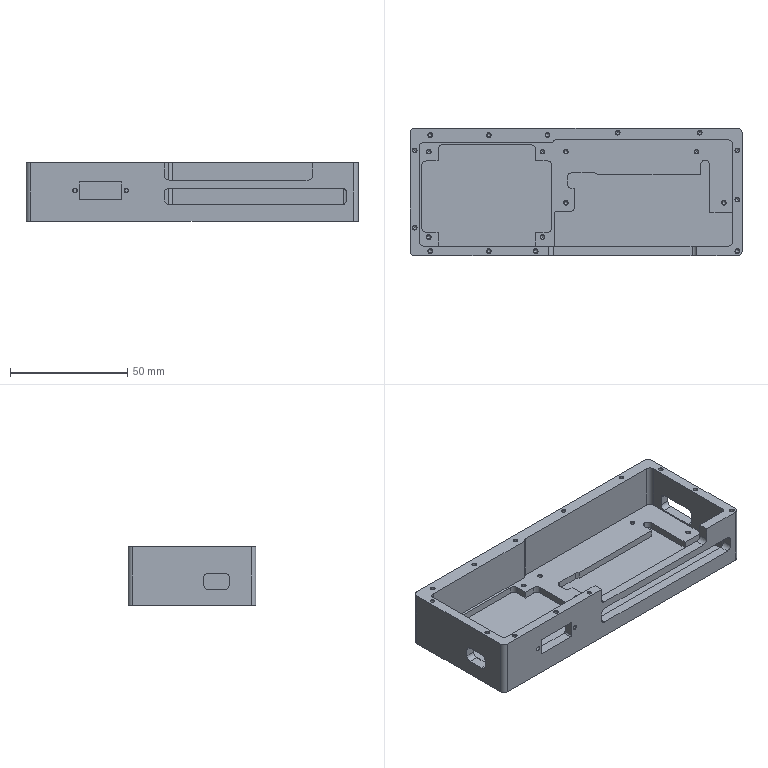Part | STEP file | Control module cavity | 1 solid | 186 faces | box 141.709 x 54.52 x 25 mm | volume 59399 mm3 | cylinder 72 | plane 60 | cone 54 | commonest cylinder face diameters 4 x36 1.6 x23 1 x4 2.5 x4 2 x3 2.54 x2